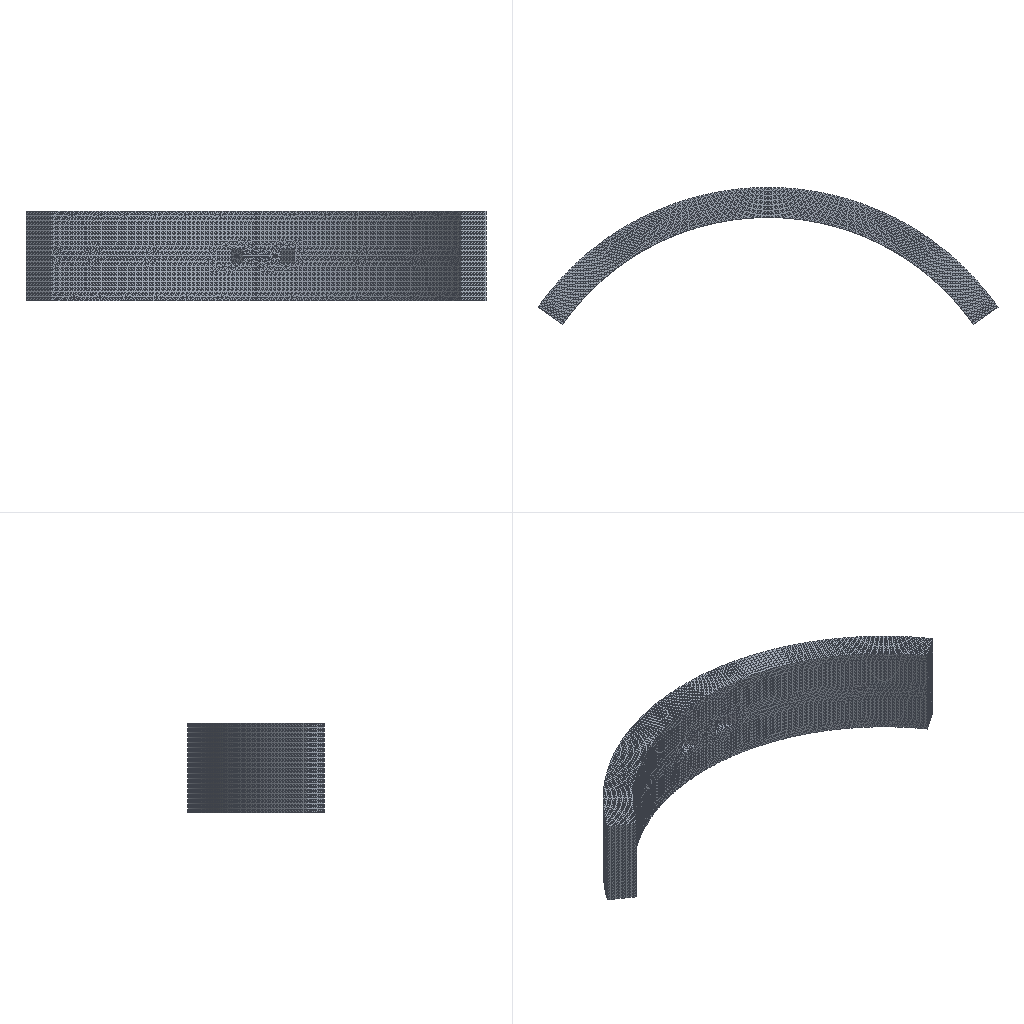Simulation study | abaqus
Set-up summary:
category,name,step,type,value,unit,region
solver,abaqus
solver,version,,,Abaqus/Standard 2020
units,not stated in the deck,,not stated
analysis,deck,,static,static
load_step,Step-1,Step-1,static
load_step,Step-2,Step-2,static
load_step,requested,,,2
mesh,nodes,,,33958
mesh,elements,,,173630
element_type,C3D4,,solid,173630
load,load commands in deck,,count,4
bc,support commands in deck,,count,2
material,GUANPIAN,,in results
material,LUOSHUAN,,in results
check,setup vs results,,match,"per instance, exact: element labels, types and connectivity; labels of the nodes the elements use; coordinates not compared"
Abaqus input file, long lists of numbers shortened:
*Heading
** Job name: Job-1 Model name: Model-1
** Generated by: Abaqus/CAE 2020
*Preprint, echo=NO, model=NO, history=NO, contact=NO
**
** PARTS
**
*Part, name=Part-1
*Node
      1,   5415.547,    6910.075,         600.
      2,   2137.132,    6910.075,         600.
** (16475 more lines like these left out)
*Element, type=C3D4
    1, 6673, 6674, 6675, 6676
    2, 6673, 6674, 6677, 6678
** (85075 more lines like these left out)
*Nset, nset=Set-33, generate
     1,  16477,      1
*Elset, elset=Set-33, generate
     1,  85077,      1
** Section: Section-1
*Solid Section, elset=Set-33, material=guanpian
,
*End Part
**
*Part, name=luoshuan
*Node
      1,   1815.458,  -103.665,   603.43
      2,   1794.725,  -75.309,    565.088
** (1002 more lines like these left out)
*Element, type=C3D4
  1, 842, 843, 844, 845
  2, 842, 846,  47,   7
** (3474 more lines like these left out)
*Nset, nset=Set-3, generate
    1,  1004,     1
*Elset, elset=Set-3, generate
    1,  3476,     1
** Section: Section-2
*Solid Section, elset=Set-3, material=luoshuan
,
*End Part
**
**
** ASSEMBLY
**
*Assembly, name=Assembly
**
*Instance, name=Part-1-1, part=Part-1
1131.228, -7001.414,        -600.
1131.228, -7001.414,        -600., 1131.228, -7001.414, -599., 27.5
*End Instance
**
*Instance, name=luoshuan-1, part=luoshuan
2639.383, 121.344, -1266.961
2639.383, 121.344, -1266.961, 2640.007, 121.614, -1266.228, 146.146
*End Instance
**
*Instance, name=Part-1-2, part=Part-1
4357.09, -7001.414,         600.
4357.09, -7001.414,         600., 4357.328, -7000.443,         600.,         180.
*End Instance
**
*Nset, nset=view, instance=Part-1-1
     1,     2,     5,     8,     9,    12,    13,    14,    16,    17,    20,    21,    22,    27,    28,    29
    30,    31,    32,    33,    34,    35,    36,    37,    38,    39,    40,    41,    42,    43,    44,    45
** (535 more lines like these left out)
*Nset, nset=view, instance=Part-1-2
     1,     2,     3,     4,     5,     6,     7,     8,     9,    10,    11,    12,    13,    14,    15,    16
    17,    18,    19,    20,    21,    22,    23,    24,    25,    26,    39,    40,    41,    42,    43,    44
** (532 more lines like these left out)
*Elset, elset=view, instance=Part-1-1, generate
 42430,  85077,      1
*Elset, elset=view, instance=Part-1-2, generate
     1,  42429,      1
*Nset, nset=_PickedSet80, internal, instance=Part-1-1
  19,  20,  38, 475, 476, 477, 478, 479, 480, 481, 482, 483, 484, 485, 853, 854
 855, 856, 857, 858, 859, 860, 861, 862, 863
*Elset, elset=_PickedSet80, internal, instance=Part-1-1
 25635, 26637, 27583, 31694, 31700, 31977, 31996, 32044, 32049, 32075, 32106, 32123, 32966, 35600, 35681, 35690
 35691, 35716, 36707, 37493, 39038, 40121, 41618, 42349, 67122, 68713, 68737, 69302, 69567, 69861, 70430, 70744
** (1 more lines like these left out)
*Nset, nset=_PickedSet81, internal, instance=Part-1-2
  19,  20,  38, 475, 476, 477, 478, 479, 480, 481, 482, 483, 484, 485, 853, 854
 855, 856, 857, 858, 859, 860, 861, 862, 863
*Elset, elset=_PickedSet81, internal, instance=Part-1-2
 25635, 26637, 27583, 31694, 31700, 31977, 31996, 32044, 32049, 32075, 32106, 32123, 32966, 35600, 35681, 35690
 35691, 35716, 36707, 37493, 39038, 40121, 41618, 42349, 67122, 68713, 68737, 69302, 69567, 69861, 70430, 70744
** (1 more lines like these left out)
*Nset, nset=_PickedSet103, internal, instance=Part-1-1
 2,
*Nset, nset=_PickedSet104, internal, instance=Part-1-2
 2,
*Elset, elset=_guanbi1_S3, internal, instance=Part-1-1
  1733,  2302,  2543,  2545,  2772,  3009,  3874,  4199,  4485,  4488,  4502,  5110,  5409,  6025,  6030,  6031
  6354,  7042,  7786,  8218,  8812,  9035,  9448,  9452,  9453,  9480,  9487,  9513,  9524,  9529,  9536,  9540
** (22 more lines like these left out)
*Elset, elset=_guanbi1_S2, internal, instance=Part-1-1
 26650, 29690, 29876, 30021, 30068, 37006, 50150, 68057, 69025, 69324, 70166, 74141, 74175, 74367, 77222
*Elset, elset=_guanbi1_S4, internal, instance=Part-1-1
 21875, 26347, 26956, 27272, 28262, 29859, 29877, 30628, 33440, 36799, 37530, 38724, 40352, 41085, 41266, 65047
 65049, 67890, 69003, 69036, 73745, 74158, 74213, 74358, 82247
*Elset, elset=_guanbi1_S1, internal, instance=Part-1-1
 24035, 24852, 25720, 27267, 29454, 29558, 29829, 67005, 67266, 67805, 69043, 70761, 72410, 73373, 74197, 74212
 75607,
*Surface, type=ELEMENT, name=guanbi1
_guanbi1_S3, S3
_guanbi1_S2, S2
_guanbi1_S4, S4
_guanbi1_S1, S1
*Elset, elset=_guanbi2_S3, internal, instance=Part-1-2
  1733,  2302,  2543,  2545,  2772,  3009,  3874,  4199,  4485,  4488,  4502,  5110,  5409,  6025,  6030,  6031
  6354,  7042,  7786,  8218,  8812,  9035,  9448,  9452,  9453,  9480,  9487,  9513,  9524,  9529,  9536,  9540
** (22 more lines like these left out)
*Elset, elset=_guanbi2_S2, internal, instance=Part-1-2
 26650, 29690, 29876, 30021, 30068, 37006, 50150, 68057, 69025, 69324, 70166, 74141, 74175, 74367, 77222
*Elset, elset=_guanbi2_S4, internal, instance=Part-1-2
 21875, 26347, 26956, 27272, 28262, 29859, 29877, 30628, 33440, 36799, 37530, 38724, 40352, 41085, 41266, 65047
 65049, 67890, 69003, 69036, 73745, 74158, 74213, 74358, 82247
*Elset, elset=_guanbi2_S1, internal, instance=Part-1-2
 24035, 24852, 25720, 27267, 29454, 29558, 29829, 67005, 67266, 67805, 69043, 70761, 72410, 73373, 74197, 74212
 75607,
*Surface, type=ELEMENT, name=guanbi2
_guanbi2_S3, S3
_guanbi2_S2, S2
_guanbi2_S4, S4
_guanbi2_S1, S1
*Elset, elset=_luokong_S4, internal, instance=Part-1-1
 29361, 29420, 29453, 29455, 32522, 33797, 37242, 65040, 65712, 67635, 67677, 74156
*Elset, elset=_luokong_S4, internal, instance=Part-1-2
 29361, 29420, 29453, 29455, 32522, 33797, 37242, 65040, 65712, 67635, 67677, 74156
*Elset, elset=_luokong_S3, internal, instance=Part-1-1
 22071, 24667, 24673, 24815, 24830, 24834, 24836, 24950, 24984, 25735, 29349, 29409, 29410, 29416, 29444, 29448
 29464, 29478, 29492, 29497, 29512, 29517, 29528, 29536, 29555, 29558, 29571, 29572, 29574, 29610, 29621, 29631
** (3 more lines like these left out)
*Elset, elset=_luokong_S3, internal, instance=Part-1-2
 22071, 24667, 24673, 24815, 24830, 24834, 24836, 24950, 24984, 25735, 29349, 29409, 29410, 29416, 29444, 29448
 29464, 29478, 29492, 29497, 29512, 29517, 29528, 29536, 29555, 29558, 29571, 29572, 29574, 29610, 29621, 29631
** (3 more lines like these left out)
*Elset, elset=_luokong_S1, internal, instance=Part-1-1
 24814, 29430, 36988, 40421, 67615, 67783, 76410
*Elset, elset=_luokong_S1, internal, instance=Part-1-2
 24814, 29430, 36988, 40421, 67615, 67783, 76410
*Elset, elset=_luokong_S2, internal, instance=Part-1-1
 29400, 29412, 29429, 29562, 67702, 76798
*Elset, elset=_luokong_S2, internal, instance=Part-1-2
 29400, 29412, 29429, 29562, 67702, 76798
*Surface, type=ELEMENT, name=luokong
_luokong_S4, S4
_luokong_S3, S3
_luokong_S2, S2
_luokong_S1, S1
*Elset, elset=_luomao1_S3, internal, instance=luoshuan-1
  148,  151,  190,  193,  317,  318,  320,  321,  328,  554,  820,  823,  830,  836,  840, 2630
 2636, 2695, 2697, 2844, 2858, 2859, 2943, 2945, 2955, 2966, 3361, 3408, 3437, 3442, 3443, 3445
** (1 more lines like these left out)
*Elset, elset=_luomao1_S4, internal, instance=luoshuan-1
  150,  694, 2783, 3454
*Elset, elset=_luomao1_S2, internal, instance=luoshuan-1
 335,
*Surface, type=ELEMENT, name=luomao1
_luomao1_S3, S3
_luomao1_S4, S4
_luomao1_S2, S2
*Elset, elset=_luomao2_S3, internal, instance=luoshuan-1
  946,  998, 1056, 1074, 1078, 1082, 1179, 1180, 1489, 1509, 1549, 1663, 1697, 1703, 1744, 1759
 1787, 1875, 1887, 1889, 1981, 2078, 2079, 2479, 2487, 2491, 2494, 2497, 2504, 2519, 2522
*Elset, elset=_luomao2_S4, internal, instance=luoshuan-1
 1387, 1694, 2495, 2521
*Elset, elset=_luomao2_S2, internal, instance=luoshuan-1
 1698,
*Surface, type=ELEMENT, name=luomao2
_luomao2_S3, S3
_luomao2_S4, S4
_luomao2_S2, S2
*Elset, elset=_luoshuan_S2, internal, instance=luoshuan-1
    8,   85,   96,  189,  233,  244,  278,  373,  472,  482,  487,  492,  497,  505,  508,  509
  512,  518,  524,  529,  536,  540,  547,  584,  590,  596,  599,  602,  606,  608,  610,  613
** (12 more lines like these left out)
*Elset, elset=_luoshuan_S3, internal, instance=luoshuan-1
   21,  122,  131,  142,  226,  230,  271,  272,  273,  286,  290,  291,  300,  303,  307,  311
  313,  315,  337,  342,  343,  347,  349,  353,  354,  359,  360,  362,  366,  367,  369,  375
** (41 more lines like these left out)
*Elset, elset=_luoshuan_S1, internal, instance=luoshuan-1
  110,  125,  177,  294,  344,  348,  350,  351,  363,  385,  386,  388,  393,  395,  404,  431
  434,  439,  457,  491,  498,  501,  513,  550,  551,  570,  583,  585,  592,  595,  597,  598
** (11 more lines like these left out)
*Elset, elset=_luoshuan_S4, internal, instance=luoshuan-1
  225,  252,  355,  537,  636,  680,  704,  723,  767,  777, 1304, 1510, 1704, 1705, 1921, 2220
 2247, 2874, 2899, 2942, 3306
*Surface, type=ELEMENT, name=luoshuan
_luoshuan_S2, S2
_luoshuan_S3, S3
_luoshuan_S4, S4
_luoshuan_S1, S1
*Elset, elset=_shoukong1_S1, internal, instance=Part-1-2
 24877, 27556, 27565, 29349, 29485, 36965, 65722, 80399
*Elset, elset=_shoukong1_S3, internal, instance=Part-1-2
 22254, 24871, 24884, 29348, 29363, 29364, 29374, 29422, 29680, 31807, 31808, 33471, 33818, 33819, 33877, 33886
 36967, 37002, 38117, 39194, 40224, 40424, 40612, 40617, 41889, 66917, 67287, 67395, 67469, 67507, 67508, 67514
** (2 more lines like these left out)
*Elset, elset=_shoukong1_S2, internal, instance=Part-1-2
 29621, 32139, 33830, 33856, 33876, 39201, 40426, 67582, 67926, 76371
*Elset, elset=_shoukong1_S4, internal, instance=Part-1-2
 29666, 33596, 33831, 33854, 67924, 80651
*Surface, type=ELEMENT, name=shoukong1
_shoukong1_S1, S1
_shoukong1_S3, S3
_shoukong1_S2, S2
_shoukong1_S4, S4
*Elset, elset=_shoukong2_S1, internal, instance=Part-1-1
 24877, 27556, 27565, 29349, 29485, 36965, 65722, 80399
*Elset, elset=_shoukong2_S3, internal, instance=Part-1-1
 22254, 24871, 24884, 29348, 29363, 29364, 29374, 29422, 29680, 31807, 31808, 33471, 33818, 33819, 33877, 33886
 36967, 37002, 38117, 39194, 40224, 40424, 40612, 40617, 41889, 66917, 67287, 67395, 67469, 67507, 67508, 67514
** (2 more lines like these left out)
*Elset, elset=_shoukong2_S2, internal, instance=Part-1-1
 29621, 32139, 33830, 33856, 33876, 39201, 40426, 67582, 67926, 76371
*Elset, elset=_shoukong2_S4, internal, instance=Part-1-1
 29666, 33596, 33831, 33854, 67924, 80651
*Surface, type=ELEMENT, name=shoukong2
_shoukong2_S1, S1
_shoukong2_S3, S3
_shoukong2_S2, S2
_shoukong2_S4, S4
*Elset, elset=__PickedSurf82_S3, internal, instance=Part-1-1
    81,   132,   217,   339,   553,   953,   958,   980,  1029,  1071,  1343,  1418,  1535,  1537,  1569,  1604
  1944,  2311,  2494,  2504,  2526,  2544,  2553,  2571,  2588,  2598,  2641,  2651,  2667,  2704,  2710,  2731
** (193 more lines like these left out)
*Elset, elset=__PickedSurf82_S3, internal, instance=Part-1-2
    81,   132,   217,   339,   553,   953,   958,   980,  1029,  1071,  1343,  1418,  1535,  1537,  1569,  1604
  1944,  2311,  2494,  2504,  2526,  2544,  2553,  2571,  2588,  2598,  2641,  2651,  2667,  2704,  2710,  2731
** (193 more lines like these left out)
*Elset, elset=__PickedSurf82_S4, internal, instance=Part-1-1
  2802,  4041,  4932,  5135,  5298,  5511,  5535,  5549,  6073,  6119,  6473,  6580,  7101,  8676,  8701,  9011
  9307,  9548, 10054, 10148, 10156, 10874, 11855, 12092, 12137, 12573, 12817, 12837, 12951, 13243, 13704, 13823
** (4 more lines like these left out)
*Elset, elset=__PickedSurf82_S4, internal, instance=Part-1-2
  2802,  4041,  4932,  5135,  5298,  5511,  5535,  5549,  6073,  6119,  6473,  6580,  7101,  8676,  8701,  9011
  9307,  9548, 10054, 10148, 10156, 10874, 11855, 12092, 12137, 12573, 12817, 12837, 12951, 13243, 13704, 13823
** (4 more lines like these left out)
*Elset, elset=__PickedSurf82_S2, internal, instance=Part-1-1
  2166,  3958,  3998,  4564,  5107,  5886,  5920,  5963,  6672,  6946,  8447,  8876, 10550, 10894, 11973, 12486
 12511, 12572, 12728, 12731, 12869, 13436, 13472, 14161, 14590, 14860, 15554, 15691, 17101, 17716, 44899, 46699
** (2 more lines like these left out)
*Elset, elset=__PickedSurf82_S2, internal, instance=Part-1-2
  2166,  3958,  3998,  4564,  5107,  5886,  5920,  5963,  6672,  6946,  8447,  8876, 10550, 10894, 11973, 12486
 12511, 12572, 12728, 12731, 12869, 13436, 13472, 14161, 14590, 14860, 15554, 15691, 17101, 17716, 44899, 46699
** (2 more lines like these left out)
*Elset, elset=__PickedSurf82_S1, internal, instance=Part-1-1
  5175,  5520,  7405,  8094,  9239, 11659, 12579, 14510, 14739, 15062, 15568, 16100, 19012, 20179, 21448, 45072
 47544, 48202, 48794, 52332, 54117, 54489, 55346, 58452, 60742, 61573, 63708, 64026
*Elset, elset=__PickedSurf82_S1, internal, instance=Part-1-2
  5175,  5520,  7405,  8094,  9239, 11659, 12579, 14510, 14739, 15062, 15568, 16100, 19012, 20179, 21448, 45072
 47544, 48202, 48794, 52332, 54117, 54489, 55346, 58452, 60742, 61573, 63708, 64026
*Surface, type=ELEMENT, name=_PickedSurf82, internal
__PickedSurf82_S3, S3
__PickedSurf82_S4, S4
__PickedSurf82_S2, S2
__PickedSurf82_S1, S1
*Nset, nset="_T-Datum csys-1", internal
_PickedSet103,
*Transform, nset="_T-Datum csys-1"
          0.,           0.,           1., -0.8192, 0.5736,           0.
*Nset, nset="_T-Datum csys-2", internal
_PickedSet104,
*Transform, nset="_T-Datum csys-2"
          0.,           0.,          -1., 0.8192, 0.5736,           0.
** Constraint: Constraint-1
*Tie, name=Constraint-1, adjust=yes, position tolerance=1.
luomao1, shoukong1
** Constraint: Constraint-2
*Tie, name=Constraint-2, adjust=yes, position tolerance=1.
luomao2, shoukong2
*End Assembly
**
** MATERIALS
**
*Material, name=guanpian
*Density
 2.4e-15,
*Elastic
34500., 0.2
*Material, name=luoshuan
*Elastic
210000., 0.3
**
** INTERACTION PROPERTIES
**
*Surface Interaction, name=IntProp-1
1.,
*Friction, slip tolerance=0.005
 0.3,
*Surface Behavior, pressure-overclosure=HARD
*Surface Interaction, name=IntProp-2
1.,
*Surface Behavior, pressure-overclosure=HARD
**
** INTERACTIONS
**
** Interaction: Int-1
*Contact Pair, interaction=IntProp-1, type=SURFACE TO SURFACE, adjust=5.
luoshuan, luokong
** Interaction: Int-2
*Contact Pair, interaction=IntProp-2, type=SURFACE TO SURFACE
guanbi2, guanbi1
** ----------------------------------------------------------------
**
** STEP: Step-1
**
*Step, name=Step-1, nlgeom=YES, inc=10000
*Static
0.0001, 1., 1e-20, 1.
**
** BOUNDARY CONDITIONS
**
** Name: BC-1 Type: 对称/反对称/完全固定
*Boundary
_PickedSet80, ENCASTRE
** Name: BC-2 Type: 对称/反对称/完全固定
*Boundary
_PickedSet81, XASYMM
**
** LOADS
**
** Name: Load-1   Type: Gravity
*Dload
, GRAV, 1000., 0., -1., 0.
**
** OUTPUT REQUESTS
**
*Restart, write, frequency=0
**
** FIELD OUTPUT: F-Output-1
**
*Output, field, variable=PRESELECT
**
** HISTORY OUTPUT: H-Output-1
**
*Output, history, variable=PRESELECT
*End Step
** ----------------------------------------------------------------
**
** STEP: Step-2
**
*Step, name=Step-2, nlgeom=YES, inc=100000
*Static
1e-05, 1., 1e-20, 1.
**
** LOADS
**
** Name: Load-2   Type: Surface traction
*Dsload
_PickedSurf82, TRVEC, 0.6, 6.77628e-10, -1., 0.
** Name: Load-3   Type: Concentrated force
*Cload
_PickedSet103, 3, -1170.
** Name: Load-4   Type: Concentrated force
*Cload
_PickedSet104, 3, -1170.
**
** OUTPUT REQUESTS
**
*Restart, write, frequency=0
**
** FIELD OUTPUT: F-Output-1
**
*Output, field, variable=PRESELECT
**
** HISTORY OUTPUT: H-Output-1
**
*Output, history, variable=PRESELECT
*End Step
Results summary:
result,step,,completed,increments=23 time=1.0/1.0
result,step,,completed,increments=30 time=1.0/1.0
result,analysis,,,static
result,last_loadstep,,,2
result,primary field,,,U
result,reaction total,,FX,20346.809,model units
result,reaction total,,FY,5008117.941,model units
result,reaction total,,FZ,31.438,model units